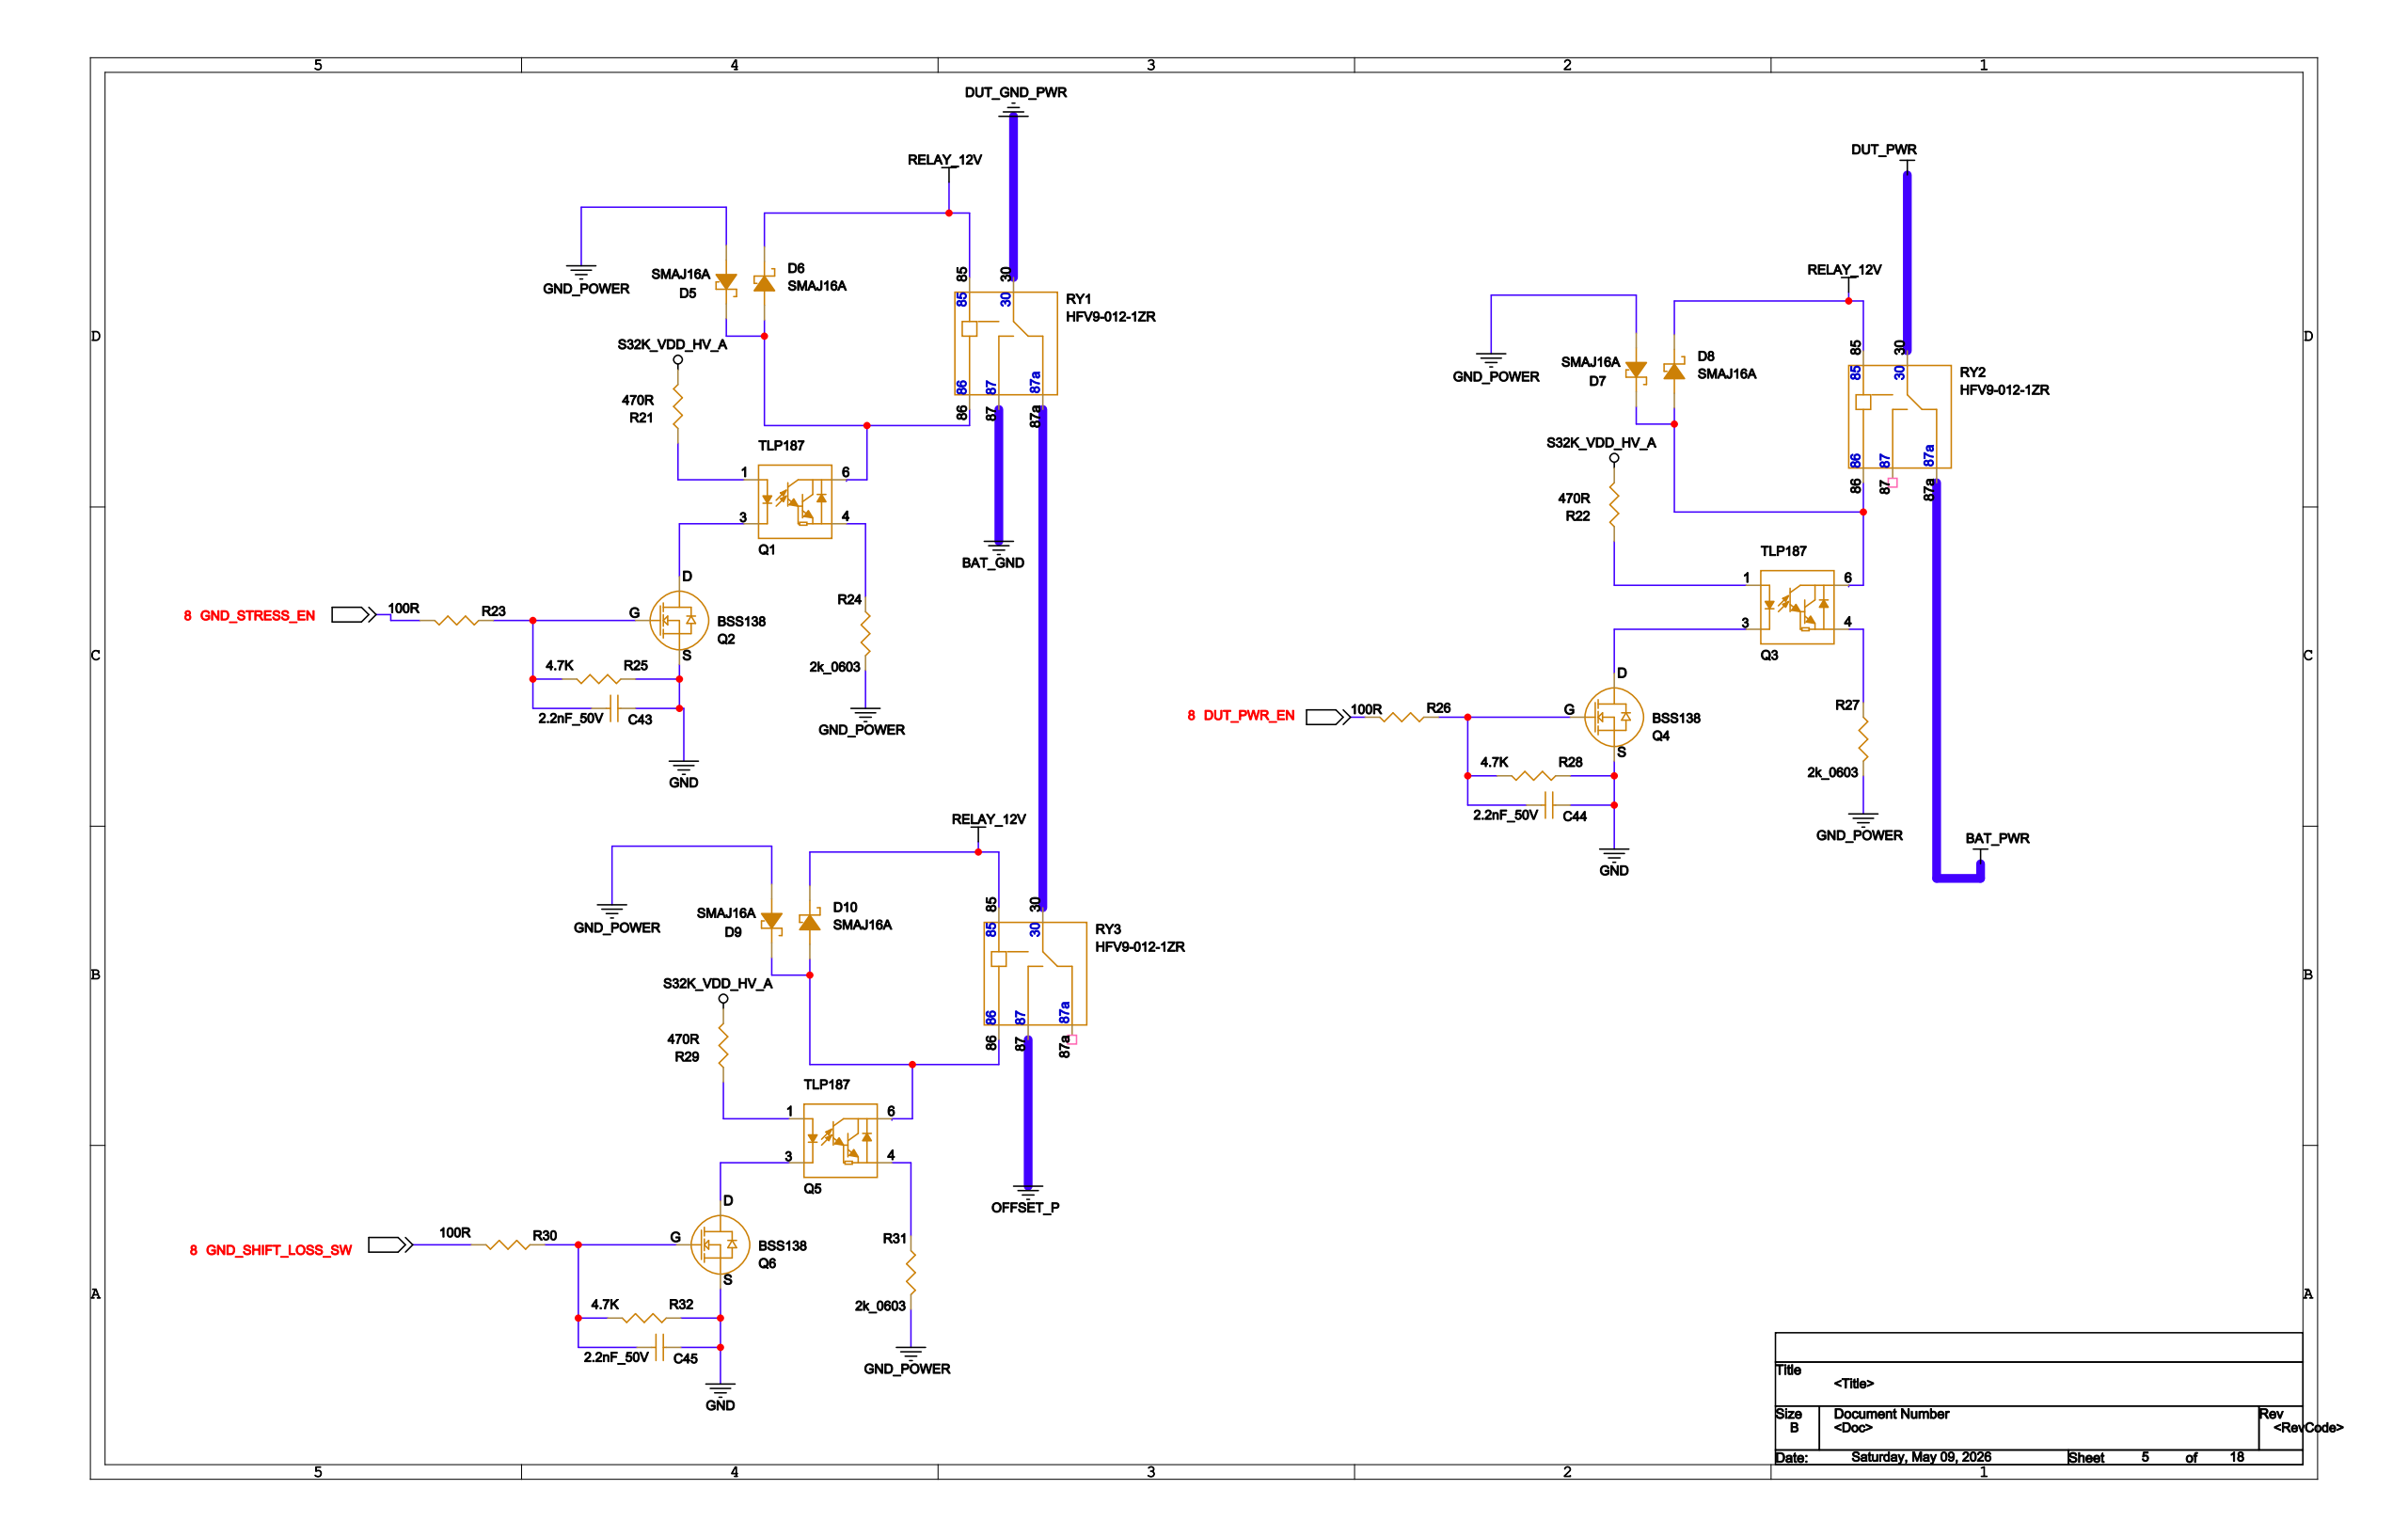Circuit board | Cadence Allegro | 330 parts | 215 nets | one sheet of the schematic
Parts on this sheet (reference | value | footprint):
C43 | 2.2nF_50V | 0603
C44 | 2.2nF_50V | 0603
C45 | 2.2nF_50V | 0603
D5 | SMAJ16A | DO-214AC
D6 | SMAJ16A | DO-214AC
D7 | SMAJ16A | DO-214AC
D8 | SMAJ16A | DO-214AC
D9 | SMAJ16A | DO-214AC
D10 | SMAJ16A | DO-214AC
Q1 | TLP187 | TLP187
Q2 | BSS138 | 003_SOT23B
Q3 | TLP187 | TLP187
Q4 | BSS138 | 003_SOT23B
Q5 | TLP187 | TLP187
Q6 | BSS138 | 003_SOT23B
R21 | 470R | 0402
R22 | 470R | 0402
R23 | 100R | 0402
R24 | 2k_0603 | 0603
R25 | 4.7K | 0402
R26 | 100R | 0402
R27 | 2k_0603 | 0603
R28 | 4.7K | 0402
R29 | 470R | 0402
R30 | 100R | 0402
R31 | 2k_0603 | 0603
R32 | 4.7K | 0402
RY1 | HFV9-012-1ZR | HFV9-012-1ZR
RY2 | HFV9-012-1ZR | HFV9-012-1ZR
RY3 | HFV9-012-1ZR | HFV9-012-1ZR
Nets of these parts (net: part-pin ...):
GND: C43-1 C44-1 C45-1 Q2-S Q4-S Q6-S R25-2 R28-2 R32-2
BAT_GND: D5-1 D7-1 D9-1 R24-2 R27-2 R31-2 RY1-87
S32K_VDD_HV_A: R21-2 R22-2 R29-2
BAT_PWR: RY2-87A
DUT_GND_PWR: RY1-30
DUT_PWR: RY2-30
OFFSET_P: RY3-87
N16898538: C44-2 Q4-G R26-2 R28-1
N16860030: C45-2 Q6-G R30-2 R32-1
N16859227: C43-2 Q2-G R23-2 R25-1
N16859160: Q1-1 R21-1
N16899729: Q3-1 R22-1
N16859963: Q5-1 R29-1
N16859192: Q1-4 R24-1
N16898502: Q3-4 R27-1
N16859995: Q5-4 R31-1
RELAY_12V: D6-2 D8-2 D10-2 RY1-85 RY2-85 RY3-85
N16859935: D9-2 D10-1 Q5-6 RY3-86
N16859132: D5-2 D6-1 Q1-6 RY1-86
N16898440: D7-2 D8-1 Q3-6 RY2-86
N16859188: Q1-3 Q2-D
N16899993: Q3-3 Q4-D
N16859991: Q5-3 Q6-D
N16860773: RY1-87A RY3-30
DUT_PWR_EN: R26-1
GND_STRESS_EN: R23-1
GND_SHIFT_LOSS_SW: R30-1